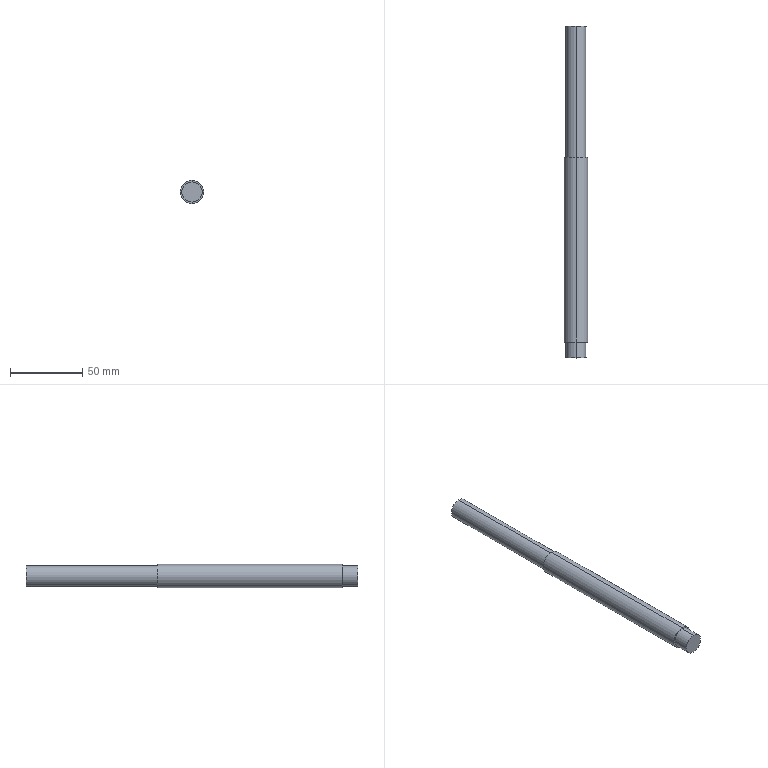Part | SolidWorks | features BaseBody 1 | 1 solid | 10 faces | box 16 x 229 x 16 mm | volume 41260 mm3 | cylinder 6 | plane 4 | commonest cylinder face diameters 14 x4 16 x2
STEP:
#1=CARTESIAN_POINT('',(57.247,567.007,-291.268));
#2=VERTEX_POINT('',#1);
#3=CARTESIAN_POINT('',(57.247,567.007,-307.268));
#4=VERTEX_POINT('',#3);
#5=CARTESIAN_POINT('',(57.247,567.007,-299.268));
#6=DIRECTION('',(0.,1.,0.));
#7=DIRECTION('',(0.,0.,1.));
#8=AXIS2_PLACEMENT_3D('',#5,#6,#7);
#9=CIRCLE('',#8,8.);
#10=EDGE_CURVE('',#2,#4,#9,.T.);
#11=ORIENTED_EDGE('',*,*,#10,.T.);
#12=CARTESIAN_POINT('',(57.247,694.507,-307.268));
#13=VERTEX_POINT('',#12);
#14=CARTESIAN_POINT('',(57.247,458.514,-307.268));
#15=DIRECTION('',(0.,1.,0.));
#16=VECTOR('',#15,1000.);
#17=LINE('',#14,#16);
#18=EDGE_CURVE('',#4,#13,#17,.T.);
#19=ORIENTED_EDGE('',*,*,#18,.T.);
#20=CARTESIAN_POINT('',(57.247,694.507,-291.268));
#21=VERTEX_POINT('',#20);
#22=CARTESIAN_POINT('',(57.247,694.507,-299.268));
#23=DIRECTION('',(0.,-1.,0.));
#24=DIRECTION('',(0.,0.,1.));
#25=AXIS2_PLACEMENT_3D('',#22,#23,#24);
#26=CIRCLE('',#25,8.);
#27=EDGE_CURVE('',#13,#21,#26,.T.);
#28=ORIENTED_EDGE('',*,*,#27,.T.);
#29=CARTESIAN_POINT('',(57.247,458.514,-291.268));
#30=DIRECTION('',(0.,1.,0.));
#31=VECTOR('',#30,1000.);
#32=LINE('',#29,#31);
#33=EDGE_CURVE('',#2,#21,#32,.T.);
#34=ORIENTED_EDGE('',*,*,#33,.F.);
#35=EDGE_LOOP('',(#11,#19,#28,#34));
#36=FACE_OUTER_BOUND('',#35,.T.);
#37=CARTESIAN_POINT('',(57.247,458.514,-299.268));
#38=DIRECTION('',(0.,1.,0.));
#39=DIRECTION('',(0.,0.,1.));
#40=AXIS2_PLACEMENT_3D('',#37,#38,#39);
#41=CYLINDRICAL_SURFACE('',#40,8.);
#42=ADVANCED_FACE('',(#36),#41,.T.);
#43=CARTESIAN_POINT('',(57.247,694.507,-292.268));
#44=VERTEX_POINT('',#43);
#45=CARTESIAN_POINT('',(57.247,694.507,-306.268));
#46=VERTEX_POINT('',#45);
#47=CARTESIAN_POINT('',(57.247,694.507,-299.268));
#48=DIRECTION('',(0.,1.,0.));
#49=DIRECTION('',(0.,0.,1.));
#50=AXIS2_PLACEMENT_3D('',#47,#48,#49);
#51=CIRCLE('',#50,7.);
#52=EDGE_CURVE('',#44,#46,#51,.T.);
#53=ORIENTED_EDGE('',*,*,#52,.T.);
#54=CARTESIAN_POINT('',(57.247,785.007,-306.268));
#55=VERTEX_POINT('',#54);
#56=CARTESIAN_POINT('',(57.247,458.514,-306.268));
#57=DIRECTION('',(0.,1.,0.));
#58=VECTOR('',#57,1000.);
#59=LINE('',#56,#58);
#60=EDGE_CURVE('',#46,#55,#59,.T.);
#61=ORIENTED_EDGE('',*,*,#60,.T.);
#62=CARTESIAN_POINT('',(57.247,785.007,-292.268));
#63=VERTEX_POINT('',#62);
#64=CARTESIAN_POINT('',(57.247,785.007,-299.268));
#65=DIRECTION('',(0.,-1.,0.));
#66=DIRECTION('',(0.,0.,1.));
#67=AXIS2_PLACEMENT_3D('',#64,#65,#66);
#68=CIRCLE('',#67,7.);
#69=EDGE_CURVE('',#55,#63,#68,.T.);
#70=ORIENTED_EDGE('',*,*,#69,.T.);
#71=CARTESIAN_POINT('',(57.247,458.514,-292.268));
#72=DIRECTION('',(0.,1.,0.));
#73=VECTOR('',#72,1000.);
#74=LINE('',#71,#73);
#75=EDGE_CURVE('',#44,#63,#74,.T.);
#76=ORIENTED_EDGE('',*,*,#75,.F.);
#77=EDGE_LOOP('',(#53,#61,#70,#76));
#78=FACE_OUTER_BOUND('',#77,.T.);
#79=CARTESIAN_POINT('',(57.247,458.514,-299.268));
#80=DIRECTION('',(0.,1.,0.));
#81=DIRECTION('',(0.,0.,1.));
#82=AXIS2_PLACEMENT_3D('',#79,#80,#81);
#83=CYLINDRICAL_SURFACE('',#82,7.);
#84=ADVANCED_FACE('',(#78),#83,.T.);
#85=CARTESIAN_POINT('',(57.247,556.007,-292.268));
#86=VERTEX_POINT('',#85);
#87=CARTESIAN_POINT('',(57.247,556.007,-306.268));
#88=VERTEX_POINT('',#87);
#89=CARTESIAN_POINT('',(57.247,556.007,-299.268));
#90=DIRECTION('',(0.,1.,0.));
#91=DIRECTION('',(0.,0.,1.));
#92=AXIS2_PLACEMENT_3D('',#89,#90,#91);
#93=CIRCLE('',#92,7.);
#94=EDGE_CURVE('',#86,#88,#93,.T.);
#95=ORIENTED_EDGE('',*,*,#94,.T.);
#96=CARTESIAN_POINT('',(57.247,567.007,-306.268));
#97=VERTEX_POINT('',#96);
#98=CARTESIAN_POINT('',(57.247,458.514,-306.268));
#99=DIRECTION('',(0.,1.,0.));
#100=VECTOR('',#99,1000.);
#101=LINE('',#98,#100);
#102=EDGE_CURVE('',#88,#97,#101,.T.);
#103=ORIENTED_EDGE('',*,*,#102,.T.);
#104=CARTESIAN_POINT('',(57.247,567.007,-292.268));
#105=VERTEX_POINT('',#104);
#106=CARTESIAN_POINT('',(57.247,567.007,-299.268));
#107=DIRECTION('',(0.,-1.,0.));
#108=DIRECTION('',(0.,0.,1.));
#109=AXIS2_PLACEMENT_3D('',#106,#107,#108);
#110=CIRCLE('',#109,7.);
#111=EDGE_CURVE('',#97,#105,#110,.T.);
#112=ORIENTED_EDGE('',*,*,#111,.T.);
#113=CARTESIAN_POINT('',(57.247,458.514,-292.268));
#114=DIRECTION('',(0.,1.,0.));
#115=VECTOR('',#114,1000.);
#116=LINE('',#113,#115);
#117=EDGE_CURVE('',#86,#105,#116,.T.);
#118=ORIENTED_EDGE('',*,*,#117,.F.);
#119=EDGE_LOOP('',(#95,#103,#112,#118));
#120=FACE_OUTER_BOUND('',#119,.T.);
#121=CARTESIAN_POINT('',(57.247,458.514,-299.268));
#122=DIRECTION('',(0.,1.,0.));
#123=DIRECTION('',(0.,0.,1.));
#124=AXIS2_PLACEMENT_3D('',#121,#122,#123);
#125=CYLINDRICAL_SURFACE('',#124,7.);
#126=ADVANCED_FACE('',(#120),#125,.T.);
#127=ORIENTED_EDGE('',*,*,#18,.F.);
#128=CARTESIAN_POINT('',(57.247,567.007,-299.268));
#129=DIRECTION('',(0.,1.,0.));
#130=DIRECTION('',(0.,0.,1.));
#131=AXIS2_PLACEMENT_3D('',#128,#129,#130);
#132=CIRCLE('',#131,8.);
#133=EDGE_CURVE('',#4,#2,#132,.T.);
#134=ORIENTED_EDGE('',*,*,#133,.T.);
#135=ORIENTED_EDGE('',*,*,#33,.T.);
#136=CARTESIAN_POINT('',(57.247,694.507,-299.268));
#137=DIRECTION('',(0.,-1.,0.));
#138=DIRECTION('',(0.,0.,1.));
#139=AXIS2_PLACEMENT_3D('',#136,#137,#138);
#140=CIRCLE('',#139,8.);
#141=EDGE_CURVE('',#21,#13,#140,.T.);
#142=ORIENTED_EDGE('',*,*,#141,.T.);
#143=EDGE_LOOP('',(#127,#134,#135,#142));
#144=FACE_OUTER_BOUND('',#143,.T.);
#145=CARTESIAN_POINT('',(57.247,458.514,-299.268));
#146=DIRECTION('',(0.,1.,0.));
#147=DIRECTION('',(0.,0.,1.));
#148=AXIS2_PLACEMENT_3D('',#145,#146,#147);
#149=CYLINDRICAL_SURFACE('',#148,8.);
#150=ADVANCED_FACE('',(#144),#149,.T.);
#151=ORIENTED_EDGE('',*,*,#52,.F.);
#152=CARTESIAN_POINT('',(57.247,694.507,-299.268));
#153=DIRECTION('',(0.,1.,0.));
#154=DIRECTION('',(0.,0.,1.));
#155=AXIS2_PLACEMENT_3D('',#152,#153,#154);
#156=CIRCLE('',#155,7.);
#157=EDGE_CURVE('',#46,#44,#156,.T.);
#158=ORIENTED_EDGE('',*,*,#157,.F.);
#159=EDGE_LOOP('',(#151,#158));
#160=FACE_BOUND('',#159,.T.);
#161=ORIENTED_EDGE('',*,*,#141,.F.);
#162=ORIENTED_EDGE('',*,*,#27,.F.);
#163=EDGE_LOOP('',(#161,#162));
#164=FACE_OUTER_BOUND('',#163,.T.);
#165=CARTESIAN_POINT('',(57.247,694.507,-289.268));
#166=DIRECTION('',(0.,-1.,0.));
#167=DIRECTION('',(0.,0.,-1.));
#168=AXIS2_PLACEMENT_3D('',#165,#166,#167);
#169=PLANE('',#168);
#170=ADVANCED_FACE('',(#160,#164),#169,.F.);
#171=CARTESIAN_POINT('',(57.247,567.007,-299.268));
#172=DIRECTION('',(0.,-1.,0.));
#173=DIRECTION('',(0.,0.,1.));
#174=AXIS2_PLACEMENT_3D('',#171,#172,#173);
#175=CIRCLE('',#174,7.);
#176=EDGE_CURVE('',#105,#97,#175,.T.);
#177=ORIENTED_EDGE('',*,*,#176,.F.);
#178=ORIENTED_EDGE('',*,*,#111,.F.);
#179=EDGE_LOOP('',(#177,#178));
#180=FACE_BOUND('',#179,.T.);
#181=ORIENTED_EDGE('',*,*,#10,.F.);
#182=ORIENTED_EDGE('',*,*,#133,.F.);
#183=EDGE_LOOP('',(#181,#182));
#184=FACE_OUTER_BOUND('',#183,.T.);
#185=CARTESIAN_POINT('',(57.247,567.007,-309.268));
#186=DIRECTION('',(0.,1.,0.));
#187=DIRECTION('',(0.,0.,1.));
#188=AXIS2_PLACEMENT_3D('',#185,#186,#187);
#189=PLANE('',#188);
#190=ADVANCED_FACE('',(#180,#184),#189,.F.);
#191=ORIENTED_EDGE('',*,*,#60,.F.);
#192=ORIENTED_EDGE('',*,*,#157,.T.);
#193=ORIENTED_EDGE('',*,*,#75,.T.);
#194=CARTESIAN_POINT('',(57.247,785.007,-299.268));
#195=DIRECTION('',(0.,-1.,0.));
#196=DIRECTION('',(0.,0.,1.));
#197=AXIS2_PLACEMENT_3D('',#194,#195,#196);
#198=CIRCLE('',#197,7.);
#199=EDGE_CURVE('',#63,#55,#198,.T.);
#200=ORIENTED_EDGE('',*,*,#199,.T.);
#201=EDGE_LOOP('',(#191,#192,#193,#200));
#202=FACE_OUTER_BOUND('',#201,.T.);
#203=CARTESIAN_POINT('',(57.247,458.514,-299.268));
#204=DIRECTION('',(0.,1.,0.));
#205=DIRECTION('',(0.,0.,1.));
#206=AXIS2_PLACEMENT_3D('',#203,#204,#205);
#207=CYLINDRICAL_SURFACE('',#206,7.);
#208=ADVANCED_FACE('',(#202),#207,.T.);
#209=ORIENTED_EDGE('',*,*,#102,.F.);
#210=CARTESIAN_POINT('',(57.247,556.007,-299.268));
#211=DIRECTION('',(0.,1.,0.));
#212=DIRECTION('',(0.,0.,1.));
#213=AXIS2_PLACEMENT_3D('',#210,#211,#212);
#214=CIRCLE('',#213,7.);
#215=EDGE_CURVE('',#88,#86,#214,.T.);
#216=ORIENTED_EDGE('',*,*,#215,.T.);
#217=ORIENTED_EDGE('',*,*,#117,.T.);
#218=ORIENTED_EDGE('',*,*,#176,.T.);
#219=EDGE_LOOP('',(#209,#216,#217,#218));
#220=FACE_OUTER_BOUND('',#219,.T.);
#221=CARTESIAN_POINT('',(57.247,458.514,-299.268));
#222=DIRECTION('',(0.,1.,0.));
#223=DIRECTION('',(0.,0.,1.));
#224=AXIS2_PLACEMENT_3D('',#221,#222,#223);
#225=CYLINDRICAL_SURFACE('',#224,7.);
#226=ADVANCED_FACE('',(#220),#225,.T.);
#227=ORIENTED_EDGE('',*,*,#199,.F.);
#228=ORIENTED_EDGE('',*,*,#69,.F.);
#229=EDGE_LOOP('',(#227,#228));
#230=FACE_OUTER_BOUND('',#229,.T.);
#231=CARTESIAN_POINT('',(57.247,785.007,-289.268));
#232=DIRECTION('',(0.,1.,0.));
#233=DIRECTION('',(0.,0.,1.));
#234=AXIS2_PLACEMENT_3D('',#231,#232,#233);
#235=PLANE('',#234);
#236=ADVANCED_FACE('',(#230),#235,.T.);
#237=ORIENTED_EDGE('',*,*,#94,.F.);
#238=ORIENTED_EDGE('',*,*,#215,.F.);
#239=EDGE_LOOP('',(#237,#238));
#240=FACE_OUTER_BOUND('',#239,.T.);
#241=CARTESIAN_POINT('',(57.247,556.007,-309.268));
#242=DIRECTION('',(0.,-1.,0.));
#243=DIRECTION('',(0.,0.,-1.));
#244=AXIS2_PLACEMENT_3D('',#241,#242,#243);
#245=PLANE('',#244);
#246=ADVANCED_FACE('',(#240),#245,.T.);
#247=CLOSED_SHELL('',(#42,#84,#126,#150,#170,#190,#208,#226,#236,#246));
#248=MANIFOLD_SOLID_BREP('',#247);
#249=CARTESIAN_POINT('',(0.,0.,0.));
#250=DIRECTION('',(0.,0.,1.));
#251=DIRECTION('',(1.,0.,0.));
#252=AXIS2_PLACEMENT_3D('',#249,#250,#251);
#253=(LENGTH_UNIT()NAMED_UNIT(*)SI_UNIT(.MILLI.,.METRE.));
#254=UNCERTAINTY_MEASURE_WITH_UNIT(LENGTH_MEASURE(0.00001),#253,'','');
#255=(NAMED_UNIT(*)PLANE_ANGLE_UNIT()SI_UNIT($,.RADIAN.));
#256=(NAMED_UNIT(*)SI_UNIT($,.STERADIAN.)SOLID_ANGLE_UNIT());
#257=(GEOMETRIC_REPRESENTATION_CONTEXT(3)GLOBAL_UNCERTAINTY_ASSIGNED_CONTEXT((#254))GLOBAL_UNIT_ASSIGNED_CONTEXT((#253,#255,#256))REPRESENTATION_CONTEXT('',''));
#258=ADVANCED_BREP_SHAPE_REPRESENTATION('',(#248,#252),#257);